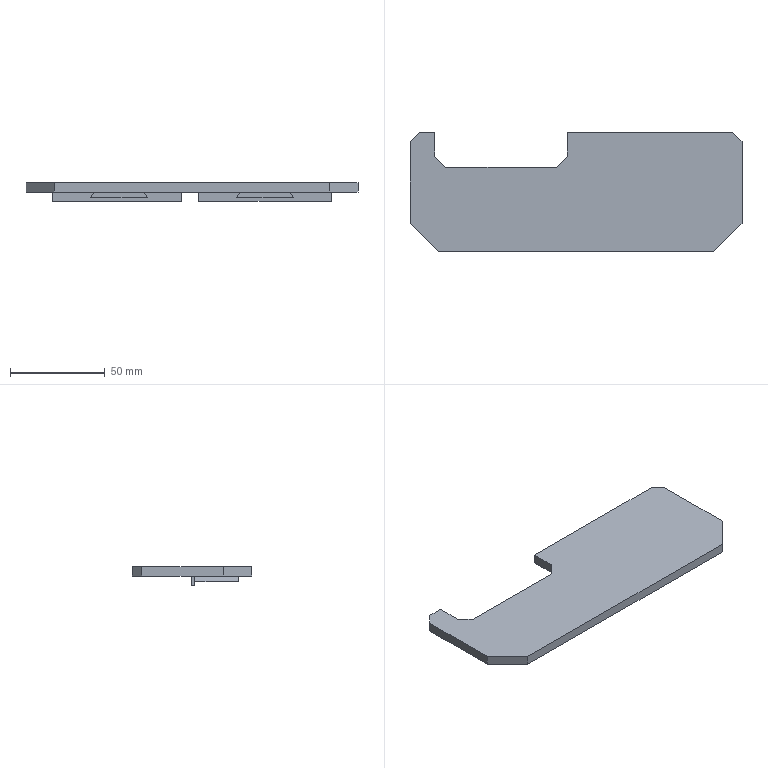Part | SolidWorks | features Chamfer 2, ICE 2, Cut 1, Extrusion 1 | 1 solid | 34 faces | box 175 x 63 x 10 mm | volume 52854 mm3 | plane 34
STEP:
#1=CARTESIAN_POINT('',(82.5,56.,0.));
#2=VERTEX_POINT('',#1);
#3=CARTESIAN_POINT('',(-4.5,56.,0.));
#4=VERTEX_POINT('',#3);
#5=CARTESIAN_POINT('',(-87.5,56.,0.));
#6=DIRECTION('',(-1.,0.,0.));
#7=VECTOR('',#6,1000.);
#8=LINE('',#5,#7);
#9=EDGE_CURVE('',#2,#4,#8,.T.);
#10=ORIENTED_EDGE('',*,*,#9,.F.);
#11=CARTESIAN_POINT('',(87.5,51.,0.));
#12=VERTEX_POINT('',#11);
#13=CARTESIAN_POINT('',(82.5,56.,0.));
#14=DIRECTION('',(0.7071,-0.7071,0.));
#15=VECTOR('',#14,1000.);
#16=LINE('',#13,#15);
#17=EDGE_CURVE('',#2,#12,#16,.T.);
#18=ORIENTED_EDGE('',*,*,#17,.T.);
#19=CARTESIAN_POINT('',(87.5,8.,0.));
#20=VERTEX_POINT('',#19);
#21=CARTESIAN_POINT('',(87.5,56.,0.));
#22=DIRECTION('',(0.,1.,0.));
#23=VECTOR('',#22,1000.);
#24=LINE('',#21,#23);
#25=EDGE_CURVE('',#20,#12,#24,.T.);
#26=ORIENTED_EDGE('',*,*,#25,.F.);
#27=CARTESIAN_POINT('',(72.5,-7.,0.));
#28=VERTEX_POINT('',#27);
#29=CARTESIAN_POINT('',(87.5,8.,0.));
#30=DIRECTION('',(-0.7071,-0.7071,0.));
#31=VECTOR('',#30,1000.);
#32=LINE('',#29,#31);
#33=EDGE_CURVE('',#20,#28,#32,.T.);
#34=ORIENTED_EDGE('',*,*,#33,.T.);
#35=CARTESIAN_POINT('',(-72.5,-7.,0.));
#36=VERTEX_POINT('',#35);
#37=CARTESIAN_POINT('',(-87.5,-7.,0.));
#38=DIRECTION('',(1.,0.,0.));
#39=VECTOR('',#38,1000.);
#40=LINE('',#37,#39);
#41=EDGE_CURVE('',#36,#28,#40,.T.);
#42=ORIENTED_EDGE('',*,*,#41,.F.);
#43=CARTESIAN_POINT('',(-87.5,8.,0.));
#44=VERTEX_POINT('',#43);
#45=CARTESIAN_POINT('',(-72.5,-7.,0.));
#46=DIRECTION('',(-0.7071,0.7071,0.));
#47=VECTOR('',#46,1000.);
#48=LINE('',#45,#47);
#49=EDGE_CURVE('',#36,#44,#48,.T.);
#50=ORIENTED_EDGE('',*,*,#49,.T.);
#51=CARTESIAN_POINT('',(-87.5,51.,0.));
#52=VERTEX_POINT('',#51);
#53=CARTESIAN_POINT('',(-87.5,56.,0.));
#54=DIRECTION('',(0.,-1.,0.));
#55=VECTOR('',#54,1000.);
#56=LINE('',#53,#55);
#57=EDGE_CURVE('',#52,#44,#56,.T.);
#58=ORIENTED_EDGE('',*,*,#57,.F.);
#59=CARTESIAN_POINT('',(-82.5,56.,0.));
#60=VERTEX_POINT('',#59);
#61=CARTESIAN_POINT('',(-87.5,51.,0.));
#62=DIRECTION('',(0.7071,0.7071,0.));
#63=VECTOR('',#62,1000.);
#64=LINE('',#61,#63);
#65=EDGE_CURVE('',#52,#60,#64,.T.);
#66=ORIENTED_EDGE('',*,*,#65,.T.);
#67=CARTESIAN_POINT('',(-74.5,56.,0.));
#68=VERTEX_POINT('',#67);
#69=CARTESIAN_POINT('',(-87.5,56.,0.));
#70=DIRECTION('',(-1.,0.,0.));
#71=VECTOR('',#70,1000.);
#72=LINE('',#69,#71);
#73=EDGE_CURVE('',#68,#60,#72,.T.);
#74=ORIENTED_EDGE('',*,*,#73,.F.);
#75=CARTESIAN_POINT('',(-74.5,43.379,0.));
#76=VERTEX_POINT('',#75);
#77=CARTESIAN_POINT('',(-74.5,56.,0.));
#78=DIRECTION('',(0.,1.,0.));
#79=VECTOR('',#78,1000.);
#80=LINE('',#77,#79);
#81=EDGE_CURVE('',#76,#68,#80,.T.);
#82=ORIENTED_EDGE('',*,*,#81,.F.);
#83=CARTESIAN_POINT('',(-68.621,37.5,0.));
#84=VERTEX_POINT('',#83);
#85=CARTESIAN_POINT('',(-74.5,43.379,0.));
#86=DIRECTION('',(-0.7071,0.7071,0.));
#87=VECTOR('',#86,1000.);
#88=LINE('',#85,#87);
#89=EDGE_CURVE('',#84,#76,#88,.T.);
#90=ORIENTED_EDGE('',*,*,#89,.F.);
#91=CARTESIAN_POINT('',(-10.379,37.5,0.));
#92=VERTEX_POINT('',#91);
#93=CARTESIAN_POINT('',(-68.621,37.5,0.));
#94=DIRECTION('',(-1.,0.,0.));
#95=VECTOR('',#94,1000.);
#96=LINE('',#93,#95);
#97=EDGE_CURVE('',#92,#84,#96,.T.);
#98=ORIENTED_EDGE('',*,*,#97,.F.);
#99=CARTESIAN_POINT('',(-4.5,43.379,0.));
#100=VERTEX_POINT('',#99);
#101=CARTESIAN_POINT('',(-10.379,37.5,0.));
#102=DIRECTION('',(-0.7071,-0.7071,0.));
#103=VECTOR('',#102,1000.);
#104=LINE('',#101,#103);
#105=EDGE_CURVE('',#100,#92,#104,.T.);
#106=ORIENTED_EDGE('',*,*,#105,.F.);
#107=CARTESIAN_POINT('',(-4.5,43.379,0.));
#108=DIRECTION('',(0.,-1.,0.));
#109=VECTOR('',#108,1000.);
#110=LINE('',#107,#109);
#111=EDGE_CURVE('',#4,#100,#110,.T.);
#112=ORIENTED_EDGE('',*,*,#111,.F.);
#113=EDGE_LOOP('',(#10,#18,#26,#34,#42,#50,#58,#66,#74,#82,#90,#98,#106,#112));
#114=FACE_OUTER_BOUND('',#113,.T.);
#115=CARTESIAN_POINT('',(-73.5,23.,0.));
#116=VERTEX_POINT('',#115);
#117=CARTESIAN_POINT('',(-73.5,25.,0.));
#118=VERTEX_POINT('',#117);
#119=CARTESIAN_POINT('',(-73.5,23.,0.));
#120=DIRECTION('',(0.,1.,0.));
#121=VECTOR('',#120,1000.);
#122=LINE('',#119,#121);
#123=EDGE_CURVE('',#116,#118,#122,.T.);
#124=ORIENTED_EDGE('',*,*,#123,.F.);
#125=CARTESIAN_POINT('',(-51.768,23.,0.));
#126=VERTEX_POINT('',#125);
#127=CARTESIAN_POINT('',(-73.5,23.,0.));
#128=DIRECTION('',(1.,0.,0.));
#129=VECTOR('',#128,1000.);
#130=LINE('',#127,#129);
#131=EDGE_CURVE('',#116,#126,#130,.T.);
#132=ORIENTED_EDGE('',*,*,#131,.T.);
#133=CARTESIAN_POINT('',(-51.768,0.,0.));
#134=VERTEX_POINT('',#133);
#135=CARTESIAN_POINT('',(-51.768,25.,0.));
#136=DIRECTION('',(0.,-1.,0.));
#137=VECTOR('',#136,1000.);
#138=LINE('',#135,#137);
#139=EDGE_CURVE('',#126,#134,#138,.T.);
#140=ORIENTED_EDGE('',*,*,#139,.T.);
#141=CARTESIAN_POINT('',(-25.232,0.,0.));
#142=VERTEX_POINT('',#141);
#143=CARTESIAN_POINT('',(77.,0.,0.));
#144=DIRECTION('',(1.,0.,0.));
#145=VECTOR('',#144,1000.);
#146=LINE('',#143,#145);
#147=EDGE_CURVE('',#134,#142,#146,.T.);
#148=ORIENTED_EDGE('',*,*,#147,.T.);
#149=CARTESIAN_POINT('',(-25.232,23.,0.));
#150=VERTEX_POINT('',#149);
#151=CARTESIAN_POINT('',(-25.232,25.,0.));
#152=DIRECTION('',(0.,-1.,0.));
#153=VECTOR('',#152,1000.);
#154=LINE('',#151,#153);
#155=EDGE_CURVE('',#150,#142,#154,.T.);
#156=ORIENTED_EDGE('',*,*,#155,.F.);
#157=CARTESIAN_POINT('',(-5.5,23.,0.));
#158=VERTEX_POINT('',#157);
#159=CARTESIAN_POINT('',(-73.5,23.,0.));
#160=DIRECTION('',(1.,0.,0.));
#161=VECTOR('',#160,1000.);
#162=LINE('',#159,#161);
#163=EDGE_CURVE('',#150,#158,#162,.T.);
#164=ORIENTED_EDGE('',*,*,#163,.T.);
#165=CARTESIAN_POINT('',(-5.5,25.,0.));
#166=VERTEX_POINT('',#165);
#167=CARTESIAN_POINT('',(-5.5,23.,0.));
#168=DIRECTION('',(0.,1.,0.));
#169=VECTOR('',#168,1000.);
#170=LINE('',#167,#169);
#171=EDGE_CURVE('',#158,#166,#170,.T.);
#172=ORIENTED_EDGE('',*,*,#171,.T.);
#173=CARTESIAN_POINT('',(77.,25.,0.));
#174=DIRECTION('',(1.,0.,0.));
#175=VECTOR('',#174,1000.);
#176=LINE('',#173,#175);
#177=EDGE_CURVE('',#118,#166,#176,.T.);
#178=ORIENTED_EDGE('',*,*,#177,.F.);
#179=EDGE_LOOP('',(#124,#132,#140,#148,#156,#164,#172,#178));
#180=FACE_BOUND('',#179,.T.);
#181=CARTESIAN_POINT('',(51.768,23.,0.));
#182=VERTEX_POINT('',#181);
#183=CARTESIAN_POINT('',(73.5,23.,0.));
#184=VERTEX_POINT('',#183);
#185=CARTESIAN_POINT('',(3.5,23.,0.));
#186=DIRECTION('',(1.,0.,0.));
#187=VECTOR('',#186,1000.);
#188=LINE('',#185,#187);
#189=EDGE_CURVE('',#182,#184,#188,.T.);
#190=ORIENTED_EDGE('',*,*,#189,.T.);
#191=CARTESIAN_POINT('',(73.5,25.,0.));
#192=VERTEX_POINT('',#191);
#193=CARTESIAN_POINT('',(73.5,23.,0.));
#194=DIRECTION('',(0.,1.,0.));
#195=VECTOR('',#194,1000.);
#196=LINE('',#193,#195);
#197=EDGE_CURVE('',#184,#192,#196,.T.);
#198=ORIENTED_EDGE('',*,*,#197,.T.);
#199=CARTESIAN_POINT('',(3.5,25.,0.));
#200=VERTEX_POINT('',#199);
#201=CARTESIAN_POINT('',(77.,25.,0.));
#202=DIRECTION('',(1.,0.,0.));
#203=VECTOR('',#202,1000.);
#204=LINE('',#201,#203);
#205=EDGE_CURVE('',#200,#192,#204,.T.);
#206=ORIENTED_EDGE('',*,*,#205,.F.);
#207=CARTESIAN_POINT('',(3.5,23.,0.));
#208=VERTEX_POINT('',#207);
#209=CARTESIAN_POINT('',(3.5,23.,0.));
#210=DIRECTION('',(0.,1.,0.));
#211=VECTOR('',#210,1000.);
#212=LINE('',#209,#211);
#213=EDGE_CURVE('',#208,#200,#212,.T.);
#214=ORIENTED_EDGE('',*,*,#213,.F.);
#215=CARTESIAN_POINT('',(25.232,23.,0.));
#216=VERTEX_POINT('',#215);
#217=CARTESIAN_POINT('',(3.5,23.,0.));
#218=DIRECTION('',(1.,0.,0.));
#219=VECTOR('',#218,1000.);
#220=LINE('',#217,#219);
#221=EDGE_CURVE('',#208,#216,#220,.T.);
#222=ORIENTED_EDGE('',*,*,#221,.T.);
#223=CARTESIAN_POINT('',(25.232,0.,0.));
#224=VERTEX_POINT('',#223);
#225=CARTESIAN_POINT('',(25.232,25.,0.));
#226=DIRECTION('',(0.,-1.,0.));
#227=VECTOR('',#226,1000.);
#228=LINE('',#225,#227);
#229=EDGE_CURVE('',#216,#224,#228,.T.);
#230=ORIENTED_EDGE('',*,*,#229,.T.);
#231=CARTESIAN_POINT('',(51.768,0.,0.));
#232=VERTEX_POINT('',#231);
#233=CARTESIAN_POINT('',(77.,0.,0.));
#234=DIRECTION('',(1.,0.,0.));
#235=VECTOR('',#234,1000.);
#236=LINE('',#233,#235);
#237=EDGE_CURVE('',#224,#232,#236,.T.);
#238=ORIENTED_EDGE('',*,*,#237,.T.);
#239=CARTESIAN_POINT('',(51.768,25.,0.));
#240=DIRECTION('',(0.,-1.,0.));
#241=VECTOR('',#240,1000.);
#242=LINE('',#239,#241);
#243=EDGE_CURVE('',#182,#232,#242,.T.);
#244=ORIENTED_EDGE('',*,*,#243,.F.);
#245=EDGE_LOOP('',(#190,#198,#206,#214,#222,#230,#238,#244));
#246=FACE_BOUND('',#245,.T.);
#247=CARTESIAN_POINT('',(0.,0.,0.));
#248=DIRECTION('',(0.,0.,1.));
#249=DIRECTION('',(1.,0.,0.));
#250=AXIS2_PLACEMENT_3D('',#247,#248,#249);
#251=PLANE('',#250);
#252=ADVANCED_FACE('',(#114,#180,#246),#251,.F.);
#253=CARTESIAN_POINT('',(23.5,23.,-3.));
#254=VERTEX_POINT('',#253);
#255=CARTESIAN_POINT('',(-48.429,23.,-127.584));
#256=DIRECTION('',(0.5,0.,0.866));
#257=VECTOR('',#256,1000.);
#258=LINE('',#255,#257);
#259=EDGE_CURVE('',#254,#216,#258,.T.);
#260=ORIENTED_EDGE('',*,*,#259,.F.);
#261=CARTESIAN_POINT('',(23.5,0.,-3.));
#262=VERTEX_POINT('',#261);
#263=CARTESIAN_POINT('',(23.5,25.,-3.));
#264=DIRECTION('',(0.,-1.,0.));
#265=VECTOR('',#264,1000.);
#266=LINE('',#263,#265);
#267=EDGE_CURVE('',#254,#262,#266,.T.);
#268=ORIENTED_EDGE('',*,*,#267,.T.);
#269=CARTESIAN_POINT('',(-48.429,0.,-127.584));
#270=DIRECTION('',(0.5,0.,0.866));
#271=VECTOR('',#270,1000.);
#272=LINE('',#269,#271);
#273=EDGE_CURVE('',#262,#224,#272,.T.);
#274=ORIENTED_EDGE('',*,*,#273,.T.);
#275=ORIENTED_EDGE('',*,*,#229,.F.);
#276=EDGE_LOOP('',(#260,#268,#274,#275));
#277=FACE_OUTER_BOUND('',#276,.T.);
#278=CARTESIAN_POINT('',(-48.429,25.,-127.584));
#279=DIRECTION('',(0.866,0.,-0.5));
#280=DIRECTION('',(-0.5,0.,-0.866));
#281=AXIS2_PLACEMENT_3D('',#278,#279,#280);
#282=PLANE('',#281);
#283=ADVANCED_FACE('',(#277),#282,.F.);
#284=CARTESIAN_POINT('',(53.5,23.,-3.));
#285=VERTEX_POINT('',#284);
#286=CARTESIAN_POINT('',(53.5,0.,-3.));
#287=VERTEX_POINT('',#286);
#288=CARTESIAN_POINT('',(53.5,25.,-3.));
#289=DIRECTION('',(0.,-1.,0.));
#290=VECTOR('',#289,1000.);
#291=LINE('',#288,#290);
#292=EDGE_CURVE('',#285,#287,#291,.T.);
#293=ORIENTED_EDGE('',*,*,#292,.F.);
#294=CARTESIAN_POINT('',(144.679,23.,-160.926));
#295=DIRECTION('',(-0.5,0.,0.866));
#296=VECTOR('',#295,1000.);
#297=LINE('',#294,#296);
#298=EDGE_CURVE('',#285,#182,#297,.T.);
#299=ORIENTED_EDGE('',*,*,#298,.T.);
#300=ORIENTED_EDGE('',*,*,#243,.T.);
#301=CARTESIAN_POINT('',(144.679,0.,-160.926));
#302=DIRECTION('',(-0.5,0.,0.866));
#303=VECTOR('',#302,1000.);
#304=LINE('',#301,#303);
#305=EDGE_CURVE('',#287,#232,#304,.T.);
#306=ORIENTED_EDGE('',*,*,#305,.F.);
#307=EDGE_LOOP('',(#293,#299,#300,#306));
#308=FACE_OUTER_BOUND('',#307,.T.);
#309=CARTESIAN_POINT('',(144.679,25.,-160.926));
#310=DIRECTION('',(0.866,0.,0.5));
#311=DIRECTION('',(0.5,0.,-0.866));
#312=AXIS2_PLACEMENT_3D('',#309,#310,#311);
#313=PLANE('',#312);
#314=ADVANCED_FACE('',(#308),#313,.T.);
#315=ORIENTED_EDGE('',*,*,#267,.F.);
#316=CARTESIAN_POINT('',(77.,23.,-3.));
#317=DIRECTION('',(1.,0.,0.));
#318=VECTOR('',#317,1000.);
#319=LINE('',#316,#318);
#320=EDGE_CURVE('',#254,#285,#319,.T.);
#321=ORIENTED_EDGE('',*,*,#320,.T.);
#322=ORIENTED_EDGE('',*,*,#292,.T.);
#323=CARTESIAN_POINT('',(77.,0.,-3.));
#324=DIRECTION('',(1.,0.,0.));
#325=VECTOR('',#324,1000.);
#326=LINE('',#323,#325);
#327=EDGE_CURVE('',#262,#287,#326,.T.);
#328=ORIENTED_EDGE('',*,*,#327,.F.);
#329=EDGE_LOOP('',(#315,#321,#322,#328));
#330=FACE_OUTER_BOUND('',#329,.T.);
#331=CARTESIAN_POINT('',(77.,25.,-3.));
#332=DIRECTION('',(0.,0.,-1.));
#333=DIRECTION('',(-1.,0.,0.));
#334=AXIS2_PLACEMENT_3D('',#331,#332,#333);
#335=PLANE('',#334);
#336=ADVANCED_FACE('',(#330),#335,.T.);
#337=ORIENTED_EDGE('',*,*,#73,.T.);
#338=CARTESIAN_POINT('',(-82.5,56.,5.));
#339=VERTEX_POINT('',#338);
#340=CARTESIAN_POINT('',(-82.5,56.,5.));
#341=DIRECTION('',(0.,0.,1.));
#342=VECTOR('',#341,1000.);
#343=LINE('',#340,#342);
#344=EDGE_CURVE('',#60,#339,#343,.T.);
#345=ORIENTED_EDGE('',*,*,#344,.T.);
#346=CARTESIAN_POINT('',(-74.5,56.,5.));
#347=VERTEX_POINT('',#346);
#348=CARTESIAN_POINT('',(-87.5,56.,5.));
#349=DIRECTION('',(-1.,0.,0.));
#350=VECTOR('',#349,1000.);
#351=LINE('',#348,#350);
#352=EDGE_CURVE('',#347,#339,#351,.T.);
#353=ORIENTED_EDGE('',*,*,#352,.F.);
#354=CARTESIAN_POINT('',(-74.5,56.,-72.403));
#355=DIRECTION('',(0.,0.,1.));
#356=VECTOR('',#355,1000.);
#357=LINE('',#354,#356);
#358=EDGE_CURVE('',#68,#347,#357,.T.);
#359=ORIENTED_EDGE('',*,*,#358,.F.);
#360=EDGE_LOOP('',(#337,#345,#353,#359));
#361=FACE_OUTER_BOUND('',#360,.T.);
#362=CARTESIAN_POINT('',(-87.5,56.,5.));
#363=DIRECTION('',(0.,-1.,0.));
#364=DIRECTION('',(0.,0.,-1.));
#365=AXIS2_PLACEMENT_3D('',#362,#363,#364);
#366=PLANE('',#365);
#367=ADVANCED_FACE('',(#361),#366,.F.);
#368=CARTESIAN_POINT('',(-87.5,51.,5.));
#369=VERTEX_POINT('',#368);
#370=CARTESIAN_POINT('',(-87.5,8.,5.));
#371=VERTEX_POINT('',#370);
#372=CARTESIAN_POINT('',(-87.5,56.,5.));
#373=DIRECTION('',(0.,-1.,0.));
#374=VECTOR('',#373,1000.);
#375=LINE('',#372,#374);
#376=EDGE_CURVE('',#369,#371,#375,.T.);
#377=ORIENTED_EDGE('',*,*,#376,.F.);
#378=CARTESIAN_POINT('',(-87.5,51.,5.));
#379=DIRECTION('',(0.,0.,-1.));
#380=VECTOR('',#379,1000.);
#381=LINE('',#378,#380);
#382=EDGE_CURVE('',#369,#52,#381,.T.);
#383=ORIENTED_EDGE('',*,*,#382,.T.);
#384=ORIENTED_EDGE('',*,*,#57,.T.);
#385=CARTESIAN_POINT('',(-87.5,8.,5.));
#386=DIRECTION('',(0.,0.,1.));
#387=VECTOR('',#386,1000.);
#388=LINE('',#385,#387);
#389=EDGE_CURVE('',#44,#371,#388,.T.);
#390=ORIENTED_EDGE('',*,*,#389,.T.);
#391=EDGE_LOOP('',(#377,#383,#384,#390));
#392=FACE_OUTER_BOUND('',#391,.T.);
#393=CARTESIAN_POINT('',(-87.5,56.,5.));
#394=DIRECTION('',(1.,0.,0.));
#395=DIRECTION('',(0.,1.,0.));
#396=AXIS2_PLACEMENT_3D('',#393,#394,#395);
#397=PLANE('',#396);
#398=ADVANCED_FACE('',(#392),#397,.F.);
#399=CARTESIAN_POINT('',(-72.5,-7.,5.));
#400=VERTEX_POINT('',#399);
#401=CARTESIAN_POINT('',(72.5,-7.,5.));
#402=VERTEX_POINT('',#401);
#403=CARTESIAN_POINT('',(-87.5,-7.,5.));
#404=DIRECTION('',(1.,0.,0.));
#405=VECTOR('',#404,1000.);
#406=LINE('',#403,#405);
#407=EDGE_CURVE('',#400,#402,#406,.T.);
#408=ORIENTED_EDGE('',*,*,#407,.F.);
#409=CARTESIAN_POINT('',(-72.5,-7.,5.));
#410=DIRECTION('',(0.,0.,-1.));
#411=VECTOR('',#410,1000.);
#412=LINE('',#409,#411);
#413=EDGE_CURVE('',#400,#36,#412,.T.);
#414=ORIENTED_EDGE('',*,*,#413,.T.);
#415=ORIENTED_EDGE('',*,*,#41,.T.);
#416=CARTESIAN_POINT('',(72.5,-7.,5.));
#417=DIRECTION('',(0.,0.,1.));
#418=VECTOR('',#417,1000.);
#419=LINE('',#416,#418);
#420=EDGE_CURVE('',#28,#402,#419,.T.);
#421=ORIENTED_EDGE('',*,*,#420,.T.);
#422=EDGE_LOOP('',(#408,#414,#415,#421));
#423=FACE_OUTER_BOUND('',#422,.T.);
#424=CARTESIAN_POINT('',(-87.5,-7.,5.));
#425=DIRECTION('',(0.,1.,0.));
#426=DIRECTION('',(0.,0.,1.));
#427=AXIS2_PLACEMENT_3D('',#424,#425,#426);
#428=PLANE('',#427);
#429=ADVANCED_FACE('',(#423),#428,.F.);
#430=ORIENTED_EDGE('',*,*,#25,.T.);
#431=CARTESIAN_POINT('',(87.5,51.,5.));
#432=VERTEX_POINT('',#431);
#433=CARTESIAN_POINT('',(87.5,51.,5.));
#434=DIRECTION('',(0.,0.,1.));
#435=VECTOR('',#434,1000.);
#436=LINE('',#433,#435);
#437=EDGE_CURVE('',#12,#432,#436,.T.);
#438=ORIENTED_EDGE('',*,*,#437,.T.);
#439=CARTESIAN_POINT('',(87.5,8.,5.));
#440=VERTEX_POINT('',#439);
#441=CARTESIAN_POINT('',(87.5,56.,5.));
#442=DIRECTION('',(0.,1.,0.));
#443=VECTOR('',#442,1000.);
#444=LINE('',#441,#443);
#445=EDGE_CURVE('',#440,#432,#444,.T.);
#446=ORIENTED_EDGE('',*,*,#445,.F.);
#447=CARTESIAN_POINT('',(87.5,8.,5.));
#448=DIRECTION('',(0.,0.,-1.));
#449=VECTOR('',#448,1000.);
#450=LINE('',#447,#449);
#451=EDGE_CURVE('',#440,#20,#450,.T.);
#452=ORIENTED_EDGE('',*,*,#451,.T.);
#453=EDGE_LOOP('',(#430,#438,#446,#452));
#454=FACE_OUTER_BOUND('',#453,.T.);
#455=CARTESIAN_POINT('',(87.5,56.,5.));
#456=DIRECTION('',(-1.,0.,0.));
#457=DIRECTION('',(0.,0.,1.));
#458=AXIS2_PLACEMENT_3D('',#455,#456,#457);
#459=PLANE('',#458);
#460=ADVANCED_FACE('',(#454),#459,.F.);
#461=CARTESIAN_POINT('',(82.5,56.,5.));
#462=VERTEX_POINT('',#461);
#463=CARTESIAN_POINT('',(-4.5,56.,5.));
#464=VERTEX_POINT('',#463);
#465=CARTESIAN_POINT('',(-87.5,56.,5.));
#466=DIRECTION('',(-1.,0.,0.));
#467=VECTOR('',#466,1000.);
#468=LINE('',#465,#467);
#469=EDGE_CURVE('',#462,#464,#468,.T.);
#470=ORIENTED_EDGE('',*,*,#469,.F.);
#471=CARTESIAN_POINT('',(82.5,56.,5.));
#472=DIRECTION('',(0.,0.,-1.));
#473=VECTOR('',#472,1000.);
#474=LINE('',#471,#473);
#475=EDGE_CURVE('',#462,#2,#474,.T.);
#476=ORIENTED_EDGE('',*,*,#475,.T.);
#477=ORIENTED_EDGE('',*,*,#9,.T.);
#478=CARTESIAN_POINT('',(-4.5,56.,-72.403));
#479=DIRECTION('',(0.,0.,1.));
#480=VECTOR('',#479,1000.);
#481=LINE('',#478,#480);
#482=EDGE_CURVE('',#4,#464,#481,.T.);
#483=ORIENTED_EDGE('',*,*,#482,.T.);
#484=EDGE_LOOP('',(#470,#476,#477,#483));
#485=FACE_OUTER_BOUND('',#484,.T.);
#486=CARTESIAN_POINT('',(-87.5,56.,5.));
#487=DIRECTION('',(0.,-1.,0.));
#488=DIRECTION('',(0.,0.,-1.));
#489=AXIS2_PLACEMENT_3D('',#486,#487,#488);
#490=PLANE('',#489);
#491=ADVANCED_FACE('',(#485),#490,.F.);
#492=ORIENTED_EDGE('',*,*,#445,.T.);
#493=CARTESIAN_POINT('',(69.25,69.25,5.));
#494=DIRECTION('',(-0.7071,0.7071,0.));
#495=VECTOR('',#494,1000.);
#496=LINE('',#493,#495);
#497=EDGE_CURVE('',#432,#462,#496,.T.);
#498=ORIENTED_EDGE('',*,*,#497,.T.);
#499=ORIENTED_EDGE('',*,*,#469,.T.);
#500=CARTESIAN_POINT('',(-4.5,43.379,5.));
#501=VERTEX_POINT('',#500);
#502=CARTESIAN_POINT('',(-4.5,43.379,5.));
#503=DIRECTION('',(0.,1.,0.));
#504=VECTOR('',#503,1000.);
#505=LINE('',#502,#504);
#506=EDGE_CURVE('',#501,#464,#505,.T.);
#507=ORIENTED_EDGE('',*,*,#506,.F.);
#508=CARTESIAN_POINT('',(-10.379,37.5,5.));
#509=VERTEX_POINT('',#508);
#510=CARTESIAN_POINT('',(-10.379,37.5,5.));
#511=DIRECTION('',(0.7071,0.7071,0.));
#512=VECTOR('',#511,1000.);
#513=LINE('',#510,#512);
#514=EDGE_CURVE('',#509,#501,#513,.T.);
#515=ORIENTED_EDGE('',*,*,#514,.F.);
#516=CARTESIAN_POINT('',(-68.621,37.5,5.));
#517=VERTEX_POINT('',#516);
#518=CARTESIAN_POINT('',(-68.621,37.5,5.));
#519=DIRECTION('',(1.,0.,0.));
#520=VECTOR('',#519,1000.);
#521=LINE('',#518,#520);
#522=EDGE_CURVE('',#517,#509,#521,.T.);
#523=ORIENTED_EDGE('',*,*,#522,.F.);
#524=CARTESIAN_POINT('',(-74.5,43.379,5.));
#525=VERTEX_POINT('',#524);
#526=CARTESIAN_POINT('',(-74.5,43.379,5.));
#527=DIRECTION('',(0.7071,-0.7071,0.));
#528=VECTOR('',#527,1000.);
#529=LINE('',#526,#528);
#530=EDGE_CURVE('',#525,#517,#529,.T.);
#531=ORIENTED_EDGE('',*,*,#530,.F.);
#532=CARTESIAN_POINT('',(-74.5,56.,5.));
#533=DIRECTION('',(0.,-1.,0.));
#534=VECTOR('',#533,1000.);
#535=LINE('',#532,#534);
#536=EDGE_CURVE('',#347,#525,#535,.T.);
#537=ORIENTED_EDGE('',*,*,#536,.F.);
#538=ORIENTED_EDGE('',*,*,#352,.T.);
#539=CARTESIAN_POINT('',(-69.25,69.25,5.));
#540=DIRECTION('',(-0.7071,-0.7071,0.));
#541=VECTOR('',#540,1000.);
#542=LINE('',#539,#541);
#543=EDGE_CURVE('',#339,#369,#542,.T.);
#544=ORIENTED_EDGE('',*,*,#543,.T.);
#545=ORIENTED_EDGE('',*,*,#376,.T.);
#546=CARTESIAN_POINT('',(-39.75,-39.75,5.));
#547=DIRECTION('',(0.7071,-0.7071,0.));
#548=VECTOR('',#547,1000.);
#549=LINE('',#546,#548);
#550=EDGE_CURVE('',#371,#400,#549,.T.);
#551=ORIENTED_EDGE('',*,*,#550,.T.);
#552=ORIENTED_EDGE('',*,*,#407,.T.);
#553=CARTESIAN_POINT('',(39.75,-39.75,5.));
#554=DIRECTION('',(0.7071,0.7071,0.));
#555=VECTOR('',#554,1000.);
#556=LINE('',#553,#555);
#557=EDGE_CURVE('',#402,#440,#556,.T.);
#558=ORIENTED_EDGE('',*,*,#557,.T.);
#559=EDGE_LOOP('',(#492,#498,#499,#507,#515,#523,#531,#537,#538,#544,#545,#551,#552,#558));
#560=FACE_OUTER_BOUND('',#559,.T.);
#561=CARTESIAN_POINT('',(0.,0.,5.));
#562=DIRECTION('',(0.,0.,1.));
#563=DIRECTION('',(1.,0.,0.));
#564=AXIS2_PLACEMENT_3D('',#561,#562,#563);
#565=PLANE('',#564);
#566=ADVANCED_FACE('',(#560),#565,.T.);
#567=ORIENTED_EDGE('',*,*,#105,.T.);
#568=CARTESIAN_POINT('',(-10.379,37.5,-72.403));
#569=DIRECTION('',(0.,0.,1.));
#570=VECTOR('',#569,1000.);
#571=LINE('',#568,#570);
#572=EDGE_CURVE('',#92,#509,#571,.T.);
#573=ORIENTED_EDGE('',*,*,#572,.T.);
#574=ORIENTED_EDGE('',*,*,#514,.T.);
#575=CARTESIAN_POINT('',(-4.5,43.379,-72.403));
#576=DIRECTION('',(0.,0.,1.));
#577=VECTOR('',#576,1000.);
#578=LINE('',#575,#577);
#579=EDGE_CURVE('',#100,#501,#578,.T.);
#580=ORIENTED_EDGE('',*,*,#579,.F.);
#581=EDGE_LOOP('',(#567,#573,#574,#580));
#582=FACE_OUTER_BOUND('',#581,.T.);
#583=CARTESIAN_POINT('',(-10.379,37.5,-72.403));
#584=DIRECTION('',(0.7071,-0.7071,0.));
#585=DIRECTION('',(0.7071,0.7071,0.));
#586=AXIS2_PLACEMENT_3D('',#583,#584,#585);
#587=PLANE('',#586);
#588=ADVANCED_FACE('',(#582),#587,.F.);
#589=ORIENTED_EDGE('',*,*,#97,.T.);
#590=CARTESIAN_POINT('',(-68.621,37.5,-72.403));
#591=DIRECTION('',(0.,0.,1.));
#592=VECTOR('',#591,1000.);
#593=LINE('',#590,#592);
#594=EDGE_CURVE('',#84,#517,#593,.T.);
#595=ORIENTED_EDGE('',*,*,#594,.T.);
#596=ORIENTED_EDGE('',*,*,#522,.T.);
#597=ORIENTED_EDGE('',*,*,#572,.F.);
#598=EDGE_LOOP('',(#589,#595,#596,#597));
#599=FACE_OUTER_BOUND('',#598,.T.);
#600=CARTESIAN_POINT('',(-68.621,37.5,-72.403));
#601=DIRECTION('',(0.,-1.,0.));
#602=DIRECTION('',(0.,0.,-1.));
#603=AXIS2_PLACEMENT_3D('',#600,#601,#602);
#604=PLANE('',#603);
#605=ADVANCED_FACE('',(#599),#604,.F.);
#606=ORIENTED_EDGE('',*,*,#89,.T.);
#607=CARTESIAN_POINT('',(-74.5,43.379,-72.403));
#608=DIRECTION('',(0.,0.,1.));
#609=VECTOR('',#608,1000.);
#610=LINE('',#607,#609);
#611=EDGE_CURVE('',#76,#525,#610,.T.);
#612=ORIENTED_EDGE('',*,*,#611,.T.);
#613=ORIENTED_EDGE('',*,*,#530,.T.);
#614=ORIENTED_EDGE('',*,*,#594,.F.);
#615=EDGE_LOOP('',(#606,#612,#613,#614));
#616=FACE_OUTER_BOUND('',#615,.T.);
#617=CARTESIAN_POINT('',(-74.5,43.379,-72.403));
#618=DIRECTION('',(-0.7071,-0.7071,0.));
#619=DIRECTION('',(0.7071,-0.7071,0.));
#620=AXIS2_PLACEMENT_3D('',#617,#618,#619);
#621=PLANE('',#620);
#622=ADVANCED_FACE('',(#616),#621,.F.);
#623=ORIENTED_EDGE('',*,*,#81,.T.);
#624=ORIENTED_EDGE('',*,*,#358,.T.);
#625=ORIENTED_EDGE('',*,*,#536,.T.);
#626=ORIENTED_EDGE('',*,*,#611,.F.);
#627=EDGE_LOOP('',(#623,#624,#625,#626));
#628=FACE_OUTER_BOUND('',#627,.T.);
#629=CARTESIAN_POINT('',(-74.5,56.,-72.403));
#630=DIRECTION('',(-1.,0.,0.));
#631=DIRECTION('',(0.,0.,1.));
#632=AXIS2_PLACEMENT_3D('',#629,#630,#631);
#633=PLANE('',#632);
#634=ADVANCED_FACE('',(#628),#633,.F.);
#635=ORIENTED_EDGE('',*,*,#111,.T.);
#636=ORIENTED_EDGE('',*,*,#579,.T.);
#637=ORIENTED_EDGE('',*,*,#506,.T.);
#638=ORIENTED_EDGE('',*,*,#482,.F.);
#639=EDGE_LOOP('',(#635,#636,#637,#638));
#640=FACE_OUTER_BOUND('',#639,.T.);
#641=CARTESIAN_POINT('',(-4.5,43.379,-72.403));
#642=DIRECTION('',(1.,0.,0.));
#643=DIRECTION('',(0.,0.,-1.));
#644=AXIS2_PLACEMENT_3D('',#641,#642,#643);
#645=PLANE('',#644);
#646=ADVANCED_FACE('',(#640),#645,.F.);
#647=ORIENTED_EDGE('',*,*,#550,.F.);
#648=ORIENTED_EDGE('',*,*,#389,.F.);
#649=ORIENTED_EDGE('',*,*,#49,.F.);
#650=ORIENTED_EDGE('',*,*,#413,.F.);
#651=EDGE_LOOP('',(#647,#648,#649,#650));
#652=FACE_OUTER_BOUND('',#651,.T.);
#653=CARTESIAN_POINT('',(-72.5,-7.,5.));
#654=DIRECTION('',(0.7071,0.7071,0.));
#655=DIRECTION('',(0.,0.,-1.));
#656=AXIS2_PLACEMENT_3D('',#653,#654,#655);
#657=PLANE('',#656);
#658=ADVANCED_FACE('',(#652),#657,.F.);
#659=ORIENTED_EDGE('',*,*,#557,.F.);
#660=ORIENTED_EDGE('',*,*,#420,.F.);
#661=ORIENTED_EDGE('',*,*,#33,.F.);
#662=ORIENTED_EDGE('',*,*,#451,.F.);
#663=EDGE_LOOP('',(#659,#660,#661,#662));
#664=FACE_OUTER_BOUND('',#663,.T.);
#665=CARTESIAN_POINT('',(87.5,8.,5.));
#666=DIRECTION('',(-0.7071,0.7071,0.));
#667=DIRECTION('',(0.,0.,-1.));
#668=AXIS2_PLACEMENT_3D('',#665,#666,#667);
#669=PLANE('',#668);
#670=ADVANCED_FACE('',(#664),#669,.F.);
#671=ORIENTED_EDGE('',*,*,#497,.F.);
#672=ORIENTED_EDGE('',*,*,#437,.F.);
#673=ORIENTED_EDGE('',*,*,#17,.F.);
#674=ORIENTED_EDGE('',*,*,#475,.F.);
#675=EDGE_LOOP('',(#671,#672,#673,#674));
#676=FACE_OUTER_BOUND('',#675,.T.);
#677=CARTESIAN_POINT('',(82.5,56.,5.));
#678=DIRECTION('',(-0.7071,-0.7071,0.));
#679=DIRECTION('',(0.,0.,-1.));
#680=AXIS2_PLACEMENT_3D('',#677,#678,#679);
#681=PLANE('',#680);
#682=ADVANCED_FACE('',(#676),#681,.F.);
#683=ORIENTED_EDGE('',*,*,#543,.F.);
#684=ORIENTED_EDGE('',*,*,#344,.F.);
#685=ORIENTED_EDGE('',*,*,#65,.F.);
#686=ORIENTED_EDGE('',*,*,#382,.F.);
#687=EDGE_LOOP('',(#683,#684,#685,#686));
#688=FACE_OUTER_BOUND('',#687,.T.);
#689=CARTESIAN_POINT('',(-87.5,51.,5.));
#690=DIRECTION('',(0.7071,-0.7071,0.));
#691=DIRECTION('',(0.,0.,-1.));
#692=AXIS2_PLACEMENT_3D('',#689,#690,#691);
#693=PLANE('',#692);
#694=ADVANCED_FACE('',(#688),#693,.F.);
#695=CARTESIAN_POINT('',(3.5,25.,-5.));
#696=VERTEX_POINT('',#695);
#697=CARTESIAN_POINT('',(3.5,25.,-5.));
#698=DIRECTION('',(0.,0.,1.));
#699=VECTOR('',#698,1000.);
#700=LINE('',#697,#699);
#701=EDGE_CURVE('',#696,#200,#700,.T.);
#702=ORIENTED_EDGE('',*,*,#701,.T.);
#703=ORIENTED_EDGE('',*,*,#205,.T.);
#704=CARTESIAN_POINT('',(73.5,25.,-5.));
#705=VERTEX_POINT('',#704);
#706=CARTESIAN_POINT('',(73.5,25.,0.));
#707=DIRECTION('',(0.,0.,-1.));
#708=VECTOR('',#707,1000.);
#709=LINE('',#706,#708);
#710=EDGE_CURVE('',#192,#705,#709,.T.);
#711=ORIENTED_EDGE('',*,*,#710,.T.);
#712=CARTESIAN_POINT('',(73.5,25.,-5.));
#713=DIRECTION('',(-1.,0.,0.));
#714=VECTOR('',#713,1000.);
#715=LINE('',#712,#714);
#716=EDGE_CURVE('',#705,#696,#715,.T.);
#717=ORIENTED_EDGE('',*,*,#716,.T.);
#718=EDGE_LOOP('',(#702,#703,#711,#717));
#719=FACE_OUTER_BOUND('',#718,.T.);
#720=CARTESIAN_POINT('',(0.,25.,0.));
#721=DIRECTION('',(0.,1.,0.));
#722=DIRECTION('',(-1.,0.,0.));
#723=AXIS2_PLACEMENT_3D('',#720,#721,#722);
#724=PLANE('',#723);
#725=ADVANCED_FACE('',(#719),#724,.T.);
#726=ORIENTED_EDGE('',*,*,#273,.F.);
#727=ORIENTED_EDGE('',*,*,#327,.T.);
#728=ORIENTED_EDGE('',*,*,#305,.T.);
#729=ORIENTED_EDGE('',*,*,#237,.F.);
#730=EDGE_LOOP('',(#726,#727,#728,#729));
#731=FACE_OUTER_BOUND('',#730,.T.);
#732=CARTESIAN_POINT('',(0.,0.,0.));
#733=DIRECTION('',(0.,1.,0.));
#734=DIRECTION('',(-1.,0.,0.));
#735=AXIS2_PLACEMENT_3D('',#732,#733,#734);
#736=PLANE('',#735);
#737=ADVANCED_FACE('',(#731),#736,.F.);
#738=CARTESIAN_POINT('',(-23.5,23.,-3.));
#739=VERTEX_POINT('',#738);
#740=CARTESIAN_POINT('',(86.929,23.,-194.268));
#741=DIRECTION('',(0.5,0.,-0.866));
#742=VECTOR('',#741,1000.);
#743=LINE('',#740,#742);
#744=EDGE_CURVE('',#150,#739,#743,.T.);
#745=ORIENTED_EDGE('',*,*,#744,.F.);
#746=ORIENTED_EDGE('',*,*,#155,.T.);
#747=CARTESIAN_POINT('',(-23.5,0.,-3.));
#748=VERTEX_POINT('',#747);
#749=CARTESIAN_POINT('',(86.929,0.,-194.268));
#750=DIRECTION('',(-0.5,0.,0.866));
#751=VECTOR('',#750,1000.);
#752=LINE('',#749,#751);
#753=EDGE_CURVE('',#748,#142,#752,.T.);
#754=ORIENTED_EDGE('',*,*,#753,.F.);
#755=CARTESIAN_POINT('',(-23.5,25.,-3.));
#756=DIRECTION('',(0.,-1.,0.));
#757=VECTOR('',#756,1000.);
#758=LINE('',#755,#757);
#759=EDGE_CURVE('',#739,#748,#758,.T.);
#760=ORIENTED_EDGE('',*,*,#759,.F.);
#761=EDGE_LOOP('',(#745,#746,#754,#760));
#762=FACE_OUTER_BOUND('',#761,.T.);
#763=CARTESIAN_POINT('',(86.929,25.,-194.268));
#764=DIRECTION('',(0.866,0.,0.5));
#765=DIRECTION('',(0.5,0.,-0.866));
#766=AXIS2_PLACEMENT_3D('',#763,#764,#765);
#767=PLANE('',#766);
#768=ADVANCED_FACE('',(#762),#767,.T.);
#769=CARTESIAN_POINT('',(-53.5,23.,-3.));
#770=VERTEX_POINT('',#769);
#771=CARTESIAN_POINT('',(-53.5,0.,-3.));
#772=VERTEX_POINT('',#771);
#773=CARTESIAN_POINT('',(-53.5,25.,-3.));
#774=DIRECTION('',(0.,-1.,0.));
#775=VECTOR('',#774,1000.);
#776=LINE('',#773,#775);
#777=EDGE_CURVE('',#770,#772,#776,.T.);
#778=ORIENTED_EDGE('',*,*,#777,.F.);
#779=CARTESIAN_POINT('',(77.,23.,-3.));
#780=DIRECTION('',(1.,0.,0.));
#781=VECTOR('',#780,1000.);
#782=LINE('',#779,#781);
#783=EDGE_CURVE('',#770,#739,#782,.T.);
#784=ORIENTED_EDGE('',*,*,#783,.T.);
#785=ORIENTED_EDGE('',*,*,#759,.T.);
#786=CARTESIAN_POINT('',(77.,0.,-3.));
#787=DIRECTION('',(-1.,0.,0.));
#788=VECTOR('',#787,1000.);
#789=LINE('',#786,#788);
#790=EDGE_CURVE('',#748,#772,#789,.T.);
#791=ORIENTED_EDGE('',*,*,#790,.T.);
#792=EDGE_LOOP('',(#778,#784,#785,#791));
#793=FACE_OUTER_BOUND('',#792,.T.);
#794=CARTESIAN_POINT('',(77.,25.,-3.));
#795=DIRECTION('',(0.,0.,1.));
#796=DIRECTION('',(1.,0.,0.));
#797=AXIS2_PLACEMENT_3D('',#794,#795,#796);
#798=PLANE('',#797);
#799=ADVANCED_FACE('',(#793),#798,.F.);
#800=ORIENTED_EDGE('',*,*,#139,.F.);
#801=CARTESIAN_POINT('',(-106.179,23.,-94.242));
#802=DIRECTION('',(-0.5,0.,-0.866));
#803=VECTOR('',#802,1000.);
#804=LINE('',#801,#803);
#805=EDGE_CURVE('',#126,#770,#804,.T.);
#806=ORIENTED_EDGE('',*,*,#805,.T.);
#807=ORIENTED_EDGE('',*,*,#777,.T.);
#808=CARTESIAN_POINT('',(-106.179,0.,-94.242));
#809=DIRECTION('',(0.5,0.,0.866));
#810=VECTOR('',#809,1000.);
#811=LINE('',#808,#810);
#812=EDGE_CURVE('',#772,#134,#811,.T.);
#813=ORIENTED_EDGE('',*,*,#812,.T.);
#814=EDGE_LOOP('',(#800,#806,#807,#813));
#815=FACE_OUTER_BOUND('',#814,.T.);
#816=CARTESIAN_POINT('',(-106.179,25.,-94.242));
#817=DIRECTION('',(0.866,0.,-0.5));
#818=DIRECTION('',(-0.5,0.,-0.866));
#819=AXIS2_PLACEMENT_3D('',#816,#817,#818);
#820=PLANE('',#819);
#821=ADVANCED_FACE('',(#815),#820,.F.);
#822=ORIENTED_EDGE('',*,*,#177,.T.);
#823=CARTESIAN_POINT('',(-5.5,25.,-5.));
#824=VERTEX_POINT('',#823);
#825=CARTESIAN_POINT('',(-5.5,25.,0.));
#826=DIRECTION('',(0.,0.,-1.));
#827=VECTOR('',#826,1000.);
#828=LINE('',#825,#827);
#829=EDGE_CURVE('',#166,#824,#828,.T.);
#830=ORIENTED_EDGE('',*,*,#829,.T.);
#831=CARTESIAN_POINT('',(-73.5,25.,-5.));
#832=VERTEX_POINT('',#831);
#833=CARTESIAN_POINT('',(-73.5,25.,-5.));
#834=DIRECTION('',(-1.,0.,0.));
#835=VECTOR('',#834,1000.);
#836=LINE('',#833,#835);
#837=EDGE_CURVE('',#824,#832,#836,.T.);
#838=ORIENTED_EDGE('',*,*,#837,.T.);
#839=CARTESIAN_POINT('',(-73.5,25.,0.));
#840=DIRECTION('',(0.,0.,1.));
#841=VECTOR('',#840,1000.);
#842=LINE('',#839,#841);
#843=EDGE_CURVE('',#832,#118,#842,.T.);
#844=ORIENTED_EDGE('',*,*,#843,.T.);
#845=EDGE_LOOP('',(#822,#830,#838,#844));
#846=FACE_OUTER_BOUND('',#845,.T.);
#847=CARTESIAN_POINT('',(0.,25.,0.));
#848=DIRECTION('',(0.,-1.,0.));
#849=DIRECTION('',(1.,0.,0.));
#850=AXIS2_PLACEMENT_3D('',#847,#848,#849);
#851=PLANE('',#850);
#852=ADVANCED_FACE('',(#846),#851,.F.);
#853=ORIENTED_EDGE('',*,*,#147,.F.);
#854=ORIENTED_EDGE('',*,*,#812,.F.);
#855=ORIENTED_EDGE('',*,*,#790,.F.);
#856=ORIENTED_EDGE('',*,*,#753,.T.);
#857=EDGE_LOOP('',(#853,#854,#855,#856));
#858=FACE_OUTER_BOUND('',#857,.T.);
#859=CARTESIAN_POINT('',(0.,0.,0.));
#860=DIRECTION('',(0.,-1.,0.));
#861=DIRECTION('',(1.,0.,0.));
#862=AXIS2_PLACEMENT_3D('',#859,#860,#861);
#863=PLANE('',#862);
#864=ADVANCED_FACE('',(#858),#863,.T.);
#865=ORIENTED_EDGE('',*,*,#843,.F.);
#866=CARTESIAN_POINT('',(-73.5,23.,-5.));
#867=VERTEX_POINT('',#866);
#868=CARTESIAN_POINT('',(-73.5,23.,-5.));
#869=DIRECTION('',(0.,1.,0.));
#870=VECTOR('',#869,1000.);
#871=LINE('',#868,#870);
#872=EDGE_CURVE('',#867,#832,#871,.T.);
#873=ORIENTED_EDGE('',*,*,#872,.F.);
#874=CARTESIAN_POINT('',(-73.5,23.,0.));
#875=DIRECTION('',(0.,0.,1.));
#876=VECTOR('',#875,1000.);
#877=LINE('',#874,#876);
#878=EDGE_CURVE('',#867,#116,#877,.T.);
#879=ORIENTED_EDGE('',*,*,#878,.T.);
#880=ORIENTED_EDGE('',*,*,#123,.T.);
#881=EDGE_LOOP('',(#865,#873,#879,#880));
#882=FACE_OUTER_BOUND('',#881,.T.);
#883=CARTESIAN_POINT('',(-73.5,23.,0.));
#884=DIRECTION('',(-1.,0.,0.));
#885=DIRECTION('',(0.,-1.,0.));
#886=AXIS2_PLACEMENT_3D('',#883,#884,#885);
#887=PLANE('',#886);
#888=ADVANCED_FACE('',(#882),#887,.T.);
#889=ORIENTED_EDGE('',*,*,#837,.F.);
#890=CARTESIAN_POINT('',(-5.5,23.,-5.));
#891=VERTEX_POINT('',#890);
#892=CARTESIAN_POINT('',(-5.5,23.,-5.));
#893=DIRECTION('',(0.,1.,0.));
#894=VECTOR('',#893,1000.);
#895=LINE('',#892,#894);
#896=EDGE_CURVE('',#891,#824,#895,.T.);
#897=ORIENTED_EDGE('',*,*,#896,.F.);
#898=CARTESIAN_POINT('',(-73.5,23.,-5.));
#899=DIRECTION('',(-1.,0.,0.));
#900=VECTOR('',#899,1000.);
#901=LINE('',#898,#900);
#902=EDGE_CURVE('',#891,#867,#901,.T.);
#903=ORIENTED_EDGE('',*,*,#902,.T.);
#904=ORIENTED_EDGE('',*,*,#872,.T.);
#905=EDGE_LOOP('',(#889,#897,#903,#904));
#906=FACE_OUTER_BOUND('',#905,.T.);
#907=CARTESIAN_POINT('',(-73.5,23.,-5.));
#908=DIRECTION('',(0.,0.,-1.));
#909=DIRECTION('',(-1.,0.,0.));
#910=AXIS2_PLACEMENT_3D('',#907,#908,#909);
#911=PLANE('',#910);
#912=ADVANCED_FACE('',(#906),#911,.T.);
#913=ORIENTED_EDGE('',*,*,#829,.F.);
#914=ORIENTED_EDGE('',*,*,#171,.F.);
#915=CARTESIAN_POINT('',(-5.5,23.,0.));
#916=DIRECTION('',(0.,0.,-1.));
#917=VECTOR('',#916,1000.);
#918=LINE('',#915,#917);
#919=EDGE_CURVE('',#158,#891,#918,.T.);
#920=ORIENTED_EDGE('',*,*,#919,.T.);
#921=ORIENTED_EDGE('',*,*,#896,.T.);
#922=EDGE_LOOP('',(#913,#914,#920,#921));
#923=FACE_OUTER_BOUND('',#922,.T.);
#924=CARTESIAN_POINT('',(-5.5,23.,0.));
#925=DIRECTION('',(1.,0.,0.));
#926=DIRECTION('',(0.,1.,0.));
#927=AXIS2_PLACEMENT_3D('',#924,#925,#926);
#928=PLANE('',#927);
#929=ADVANCED_FACE('',(#923),#928,.T.);
#930=ORIENTED_EDGE('',*,*,#163,.F.);
#931=ORIENTED_EDGE('',*,*,#744,.T.);
#932=ORIENTED_EDGE('',*,*,#783,.F.);
#933=ORIENTED_EDGE('',*,*,#805,.F.);
#934=ORIENTED_EDGE('',*,*,#131,.F.);
#935=ORIENTED_EDGE('',*,*,#878,.F.);
#936=ORIENTED_EDGE('',*,*,#902,.F.);
#937=ORIENTED_EDGE('',*,*,#919,.F.);
#938=EDGE_LOOP('',(#930,#931,#932,#933,#934,#935,#936,#937));
#939=FACE_OUTER_BOUND('',#938,.T.);
#940=CARTESIAN_POINT('',(0.,23.,0.));
#941=DIRECTION('',(0.,-1.,0.));
#942=DIRECTION('',(1.,0.,0.));
#943=AXIS2_PLACEMENT_3D('',#940,#941,#942);
#944=PLANE('',#943);
#945=ADVANCED_FACE('',(#939),#944,.T.);
#946=ORIENTED_EDGE('',*,*,#320,.F.);
#947=ORIENTED_EDGE('',*,*,#259,.T.);
#948=ORIENTED_EDGE('',*,*,#221,.F.);
#949=CARTESIAN_POINT('',(3.5,23.,-5.));
#950=VERTEX_POINT('',#949);
#951=CARTESIAN_POINT('',(3.5,23.,-5.));
#952=DIRECTION('',(0.,0.,1.));
#953=VECTOR('',#952,1000.);
#954=LINE('',#951,#953);
#955=EDGE_CURVE('',#950,#208,#954,.T.);
#956=ORIENTED_EDGE('',*,*,#955,.F.);
#957=CARTESIAN_POINT('',(73.5,23.,-5.));
#958=VERTEX_POINT('',#957);
#959=CARTESIAN_POINT('',(73.5,23.,-5.));
#960=DIRECTION('',(-1.,0.,0.));
#961=VECTOR('',#960,1000.);
#962=LINE('',#959,#961);
#963=EDGE_CURVE('',#958,#950,#962,.T.);
#964=ORIENTED_EDGE('',*,*,#963,.F.);
#965=CARTESIAN_POINT('',(73.5,23.,0.));
#966=DIRECTION('',(0.,0.,-1.));
#967=VECTOR('',#966,1000.);
#968=LINE('',#965,#967);
#969=EDGE_CURVE('',#184,#958,#968,.T.);
#970=ORIENTED_EDGE('',*,*,#969,.F.);
#971=ORIENTED_EDGE('',*,*,#189,.F.);
#972=ORIENTED_EDGE('',*,*,#298,.F.);
#973=EDGE_LOOP('',(#946,#947,#948,#956,#964,#970,#971,#972));
#974=FACE_OUTER_BOUND('',#973,.T.);
#975=CARTESIAN_POINT('',(0.,23.,0.));
#976=DIRECTION('',(0.,1.,0.));
#977=DIRECTION('',(-1.,0.,0.));
#978=AXIS2_PLACEMENT_3D('',#975,#976,#977);
#979=PLANE('',#978);
#980=ADVANCED_FACE('',(#974),#979,.F.);
#981=ORIENTED_EDGE('',*,*,#701,.F.);
#982=CARTESIAN_POINT('',(3.5,23.,-5.));
#983=DIRECTION('',(0.,1.,0.));
#984=VECTOR('',#983,1000.);
#985=LINE('',#982,#984);
#986=EDGE_CURVE('',#950,#696,#985,.T.);
#987=ORIENTED_EDGE('',*,*,#986,.F.);
#988=ORIENTED_EDGE('',*,*,#955,.T.);
#989=ORIENTED_EDGE('',*,*,#213,.T.);
#990=EDGE_LOOP('',(#981,#987,#988,#989));
#991=FACE_OUTER_BOUND('',#990,.T.);
#992=CARTESIAN_POINT('',(3.5,23.,-5.));
#993=DIRECTION('',(-1.,0.,0.));
#994=DIRECTION('',(0.,-1.,0.));
#995=AXIS2_PLACEMENT_3D('',#992,#993,#994);
#996=PLANE('',#995);
#997=ADVANCED_FACE('',(#991),#996,.T.);
#998=ORIENTED_EDGE('',*,*,#716,.F.);
#999=CARTESIAN_POINT('',(73.5,23.,-5.));
#1000=DIRECTION('',(0.,1.,0.));
#1001=VECTOR('',#1000,1000.);
#1002=LINE('',#999,#1001);
#1003=EDGE_CURVE('',#958,#705,#1002,.T.);
#1004=ORIENTED_EDGE('',*,*,#1003,.F.);
#1005=ORIENTED_EDGE('',*,*,#963,.T.);
#1006=ORIENTED_EDGE('',*,*,#986,.T.);
#1007=EDGE_LOOP('',(#998,#1004,#1005,#1006));
#1008=FACE_OUTER_BOUND('',#1007,.T.);
#1009=CARTESIAN_POINT('',(73.5,23.,-5.));
#1010=DIRECTION('',(0.,0.,-1.));
#1011=DIRECTION('',(-1.,0.,0.));
#1012=AXIS2_PLACEMENT_3D('',#1009,#1010,#1011);
#1013=PLANE('',#1012);
#1014=ADVANCED_FACE('',(#1008),#1013,.T.);
#1015=ORIENTED_EDGE('',*,*,#710,.F.);
#1016=ORIENTED_EDGE('',*,*,#197,.F.);
#1017=ORIENTED_EDGE('',*,*,#969,.T.);
#1018=ORIENTED_EDGE('',*,*,#1003,.T.);
#1019=EDGE_LOOP('',(#1015,#1016,#1017,#1018));
#1020=FACE_OUTER_BOUND('',#1019,.T.);
#1021=CARTESIAN_POINT('',(73.5,23.,0.));
#1022=DIRECTION('',(1.,0.,0.));
#1023=DIRECTION('',(0.,1.,0.));
#1024=AXIS2_PLACEMENT_3D('',#1021,#1022,#1023);
#1025=PLANE('',#1024);
#1026=ADVANCED_FACE('',(#1020),#1025,.T.);
#1027=CLOSED_SHELL('',(#252,#283,#314,#336,#367,#398,#429,#460,#491,#566,#588,#605,#622,#634,#646,#658,#670,#682,#694,#725,#737,#768,#799,#821,#852,#864,#888,#912,#929,#945,#980,#997,#1014,#1026));
#1028=MANIFOLD_SOLID_BREP('',#1027);
#1029=CARTESIAN_POINT('',(0.,0.,0.));
#1030=DIRECTION('',(0.,0.,1.));
#1031=DIRECTION('',(1.,0.,0.));
#1032=AXIS2_PLACEMENT_3D('',#1029,#1030,#1031);
#1033=(LENGTH_UNIT()NAMED_UNIT(*)SI_UNIT(.MILLI.,.METRE.));
#1034=UNCERTAINTY_MEASURE_WITH_UNIT(LENGTH_MEASURE(0.00001),#1033,'','');
#1035=(NAMED_UNIT(*)PLANE_ANGLE_UNIT()SI_UNIT($,.RADIAN.));
#1036=(NAMED_UNIT(*)SI_UNIT($,.STERADIAN.)SOLID_ANGLE_UNIT());
#1037=(GEOMETRIC_REPRESENTATION_CONTEXT(3)GLOBAL_UNCERTAINTY_ASSIGNED_CONTEXT((#1034))GLOBAL_UNIT_ASSIGNED_CONTEXT((#1033,#1035,#1036))REPRESENTATION_CONTEXT('',''));
#1038=ADVANCED_BREP_SHAPE_REPRESENTATION('',(#1028,#1032),#1037);